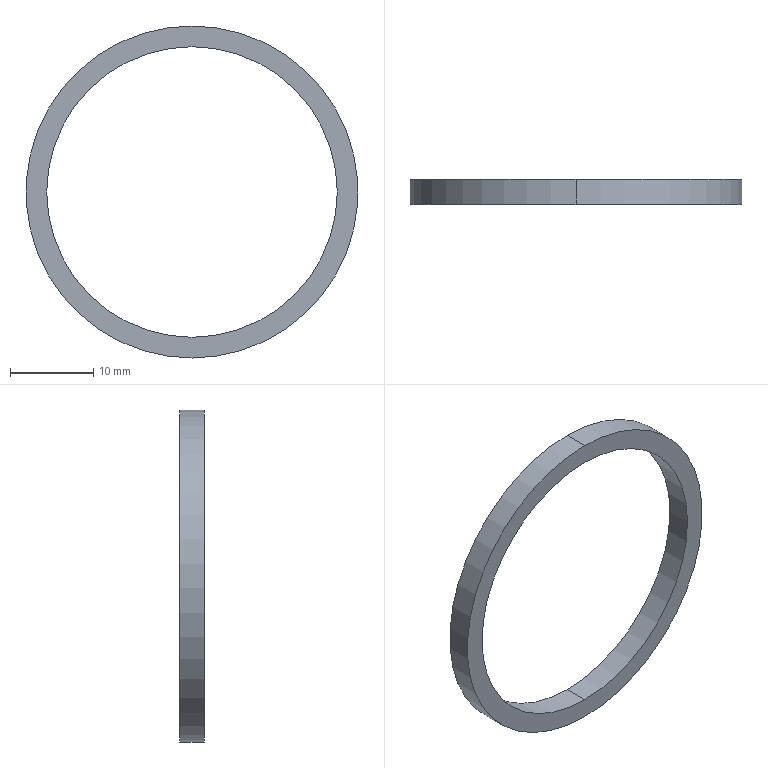Part | SolidWorks | features BaseBody 1 | 1 solid | 6 faces | box 40 x 3 x 40 mm | volume 883.573 mm3 | cylinder 4 | plane 2 | commonest cylinder face diameters 35 x2 40 x2
STEP:
#1=CARTESIAN_POINT('',(0.,1.5,17.5));
#2=VERTEX_POINT('',#1);
#3=CARTESIAN_POINT('',(0.,-1.5,17.5));
#4=VERTEX_POINT('',#3);
#5=CARTESIAN_POINT('',(0.,1.5,17.5));
#6=DIRECTION('',(0.,-1.,0.));
#7=VECTOR('',#6,1000.);
#8=LINE('',#5,#7);
#9=EDGE_CURVE('',#2,#4,#8,.T.);
#10=ORIENTED_EDGE('',*,*,#9,.F.);
#11=CARTESIAN_POINT('',(0.,1.5,-17.5));
#12=VERTEX_POINT('',#11);
#13=CARTESIAN_POINT('',(0.,1.5,0.));
#14=DIRECTION('',(0.,1.,0.));
#15=DIRECTION('',(0.,0.,1.));
#16=AXIS2_PLACEMENT_3D('',#13,#14,#15);
#17=CIRCLE('',#16,17.5);
#18=EDGE_CURVE('',#2,#12,#17,.T.);
#19=ORIENTED_EDGE('',*,*,#18,.T.);
#20=CARTESIAN_POINT('',(0.,-1.5,-17.5));
#21=VERTEX_POINT('',#20);
#22=CARTESIAN_POINT('',(0.,1.5,-17.5));
#23=DIRECTION('',(0.,-1.,0.));
#24=VECTOR('',#23,1000.);
#25=LINE('',#22,#24);
#26=EDGE_CURVE('',#12,#21,#25,.T.);
#27=ORIENTED_EDGE('',*,*,#26,.T.);
#28=CARTESIAN_POINT('',(0.,-1.5,0.));
#29=DIRECTION('',(0.,1.,0.));
#30=DIRECTION('',(0.,0.,1.));
#31=AXIS2_PLACEMENT_3D('',#28,#29,#30);
#32=CIRCLE('',#31,17.5);
#33=EDGE_CURVE('',#4,#21,#32,.T.);
#34=ORIENTED_EDGE('',*,*,#33,.F.);
#35=EDGE_LOOP('',(#10,#19,#27,#34));
#36=FACE_OUTER_BOUND('',#35,.T.);
#37=CARTESIAN_POINT('',(0.,1.5,0.));
#38=DIRECTION('',(0.,-1.,0.));
#39=DIRECTION('',(0.,0.,-1.));
#40=AXIS2_PLACEMENT_3D('',#37,#38,#39);
#41=CYLINDRICAL_SURFACE('',#40,17.5);
#42=ADVANCED_FACE('',(#36),#41,.F.);
#43=CARTESIAN_POINT('',(0.,1.5,20.));
#44=VERTEX_POINT('',#43);
#45=CARTESIAN_POINT('',(0.,-1.5,20.));
#46=VERTEX_POINT('',#45);
#47=CARTESIAN_POINT('',(0.,1.5,20.));
#48=DIRECTION('',(0.,-1.,0.));
#49=VECTOR('',#48,1000.);
#50=LINE('',#47,#49);
#51=EDGE_CURVE('',#44,#46,#50,.T.);
#52=ORIENTED_EDGE('',*,*,#51,.F.);
#53=CARTESIAN_POINT('',(0.,1.5,-20.));
#54=VERTEX_POINT('',#53);
#55=CARTESIAN_POINT('',(0.,1.5,0.));
#56=DIRECTION('',(0.,1.,0.));
#57=DIRECTION('',(0.,0.,1.));
#58=AXIS2_PLACEMENT_3D('',#55,#56,#57);
#59=CIRCLE('',#58,20.);
#60=EDGE_CURVE('',#54,#44,#59,.T.);
#61=ORIENTED_EDGE('',*,*,#60,.F.);
#62=CARTESIAN_POINT('',(0.,-1.5,-20.));
#63=VERTEX_POINT('',#62);
#64=CARTESIAN_POINT('',(0.,1.5,-20.));
#65=DIRECTION('',(0.,-1.,0.));
#66=VECTOR('',#65,1000.);
#67=LINE('',#64,#66);
#68=EDGE_CURVE('',#54,#63,#67,.T.);
#69=ORIENTED_EDGE('',*,*,#68,.T.);
#70=CARTESIAN_POINT('',(0.,-1.5,0.));
#71=DIRECTION('',(0.,1.,0.));
#72=DIRECTION('',(0.,0.,1.));
#73=AXIS2_PLACEMENT_3D('',#70,#71,#72);
#74=CIRCLE('',#73,20.);
#75=EDGE_CURVE('',#63,#46,#74,.T.);
#76=ORIENTED_EDGE('',*,*,#75,.T.);
#77=EDGE_LOOP('',(#52,#61,#69,#76));
#78=FACE_OUTER_BOUND('',#77,.T.);
#79=CARTESIAN_POINT('',(0.,1.5,0.));
#80=DIRECTION('',(0.,-1.,0.));
#81=DIRECTION('',(0.,0.,-1.));
#82=AXIS2_PLACEMENT_3D('',#79,#80,#81);
#83=CYLINDRICAL_SURFACE('',#82,20.);
#84=ADVANCED_FACE('',(#78),#83,.T.);
#85=CARTESIAN_POINT('',(0.,-1.5,0.));
#86=DIRECTION('',(0.,1.,0.));
#87=DIRECTION('',(0.,0.,1.));
#88=AXIS2_PLACEMENT_3D('',#85,#86,#87);
#89=CIRCLE('',#88,17.5);
#90=EDGE_CURVE('',#21,#4,#89,.T.);
#91=ORIENTED_EDGE('',*,*,#90,.T.);
#92=ORIENTED_EDGE('',*,*,#33,.T.);
#93=EDGE_LOOP('',(#91,#92));
#94=FACE_BOUND('',#93,.T.);
#95=ORIENTED_EDGE('',*,*,#75,.F.);
#96=CARTESIAN_POINT('',(0.,-1.5,0.));
#97=DIRECTION('',(0.,1.,0.));
#98=DIRECTION('',(0.,0.,1.));
#99=AXIS2_PLACEMENT_3D('',#96,#97,#98);
#100=CIRCLE('',#99,20.);
#101=EDGE_CURVE('',#46,#63,#100,.T.);
#102=ORIENTED_EDGE('',*,*,#101,.F.);
#103=EDGE_LOOP('',(#95,#102));
#104=FACE_OUTER_BOUND('',#103,.T.);
#105=CARTESIAN_POINT('',(0.,-1.5,0.));
#106=DIRECTION('',(0.,1.,0.));
#107=DIRECTION('',(1.,0.,0.));
#108=AXIS2_PLACEMENT_3D('',#105,#106,#107);
#109=PLANE('',#108);
#110=ADVANCED_FACE('',(#94,#104),#109,.F.);
#111=CARTESIAN_POINT('',(0.,1.5,0.));
#112=DIRECTION('',(0.,1.,0.));
#113=DIRECTION('',(0.,0.,1.));
#114=AXIS2_PLACEMENT_3D('',#111,#112,#113);
#115=CIRCLE('',#114,17.5);
#116=EDGE_CURVE('',#12,#2,#115,.T.);
#117=ORIENTED_EDGE('',*,*,#116,.F.);
#118=ORIENTED_EDGE('',*,*,#18,.F.);
#119=EDGE_LOOP('',(#117,#118));
#120=FACE_BOUND('',#119,.T.);
#121=ORIENTED_EDGE('',*,*,#60,.T.);
#122=CARTESIAN_POINT('',(0.,1.5,0.));
#123=DIRECTION('',(0.,1.,0.));
#124=DIRECTION('',(0.,0.,1.));
#125=AXIS2_PLACEMENT_3D('',#122,#123,#124);
#126=CIRCLE('',#125,20.);
#127=EDGE_CURVE('',#44,#54,#126,.T.);
#128=ORIENTED_EDGE('',*,*,#127,.T.);
#129=EDGE_LOOP('',(#121,#128));
#130=FACE_OUTER_BOUND('',#129,.T.);
#131=CARTESIAN_POINT('',(0.,1.5,0.));
#132=DIRECTION('',(0.,1.,0.));
#133=DIRECTION('',(1.,0.,0.));
#134=AXIS2_PLACEMENT_3D('',#131,#132,#133);
#135=PLANE('',#134);
#136=ADVANCED_FACE('',(#120,#130),#135,.T.);
#137=ORIENTED_EDGE('',*,*,#127,.F.);
#138=ORIENTED_EDGE('',*,*,#51,.T.);
#139=ORIENTED_EDGE('',*,*,#101,.T.);
#140=ORIENTED_EDGE('',*,*,#68,.F.);
#141=EDGE_LOOP('',(#137,#138,#139,#140));
#142=FACE_OUTER_BOUND('',#141,.T.);
#143=CARTESIAN_POINT('',(0.,1.5,0.));
#144=DIRECTION('',(0.,-1.,0.));
#145=DIRECTION('',(0.,0.,-1.));
#146=AXIS2_PLACEMENT_3D('',#143,#144,#145);
#147=CYLINDRICAL_SURFACE('',#146,20.);
#148=ADVANCED_FACE('',(#142),#147,.T.);
#149=ORIENTED_EDGE('',*,*,#116,.T.);
#150=ORIENTED_EDGE('',*,*,#9,.T.);
#151=ORIENTED_EDGE('',*,*,#90,.F.);
#152=ORIENTED_EDGE('',*,*,#26,.F.);
#153=EDGE_LOOP('',(#149,#150,#151,#152));
#154=FACE_OUTER_BOUND('',#153,.T.);
#155=CARTESIAN_POINT('',(0.,1.5,0.));
#156=DIRECTION('',(0.,-1.,0.));
#157=DIRECTION('',(0.,0.,-1.));
#158=AXIS2_PLACEMENT_3D('',#155,#156,#157);
#159=CYLINDRICAL_SURFACE('',#158,17.5);
#160=ADVANCED_FACE('',(#154),#159,.F.);
#161=CLOSED_SHELL('',(#42,#84,#110,#136,#148,#160));
#162=MANIFOLD_SOLID_BREP('',#161);
#163=CARTESIAN_POINT('',(0.,0.,0.));
#164=DIRECTION('',(0.,0.,1.));
#165=DIRECTION('',(1.,0.,0.));
#166=AXIS2_PLACEMENT_3D('',#163,#164,#165);
#167=(LENGTH_UNIT()NAMED_UNIT(*)SI_UNIT(.MILLI.,.METRE.));
#168=UNCERTAINTY_MEASURE_WITH_UNIT(LENGTH_MEASURE(0.00001),#167,'','');
#169=(NAMED_UNIT(*)PLANE_ANGLE_UNIT()SI_UNIT($,.RADIAN.));
#170=(NAMED_UNIT(*)SI_UNIT($,.STERADIAN.)SOLID_ANGLE_UNIT());
#171=(GEOMETRIC_REPRESENTATION_CONTEXT(3)GLOBAL_UNCERTAINTY_ASSIGNED_CONTEXT((#168))GLOBAL_UNIT_ASSIGNED_CONTEXT((#167,#169,#170))REPRESENTATION_CONTEXT('',''));
#172=ADVANCED_BREP_SHAPE_REPRESENTATION('',(#162,#166),#171);